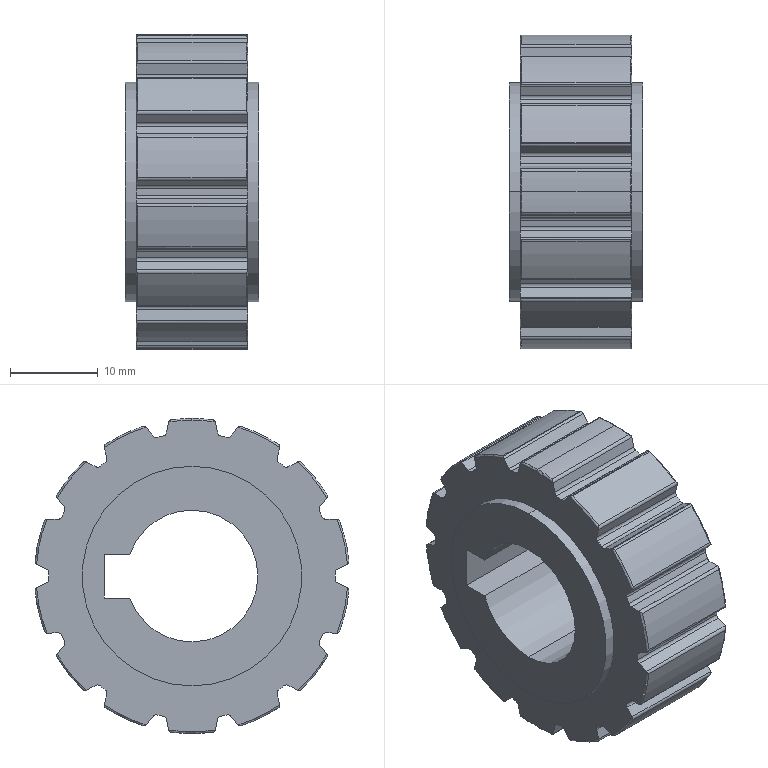Part | SolidWorks | features ICE 3, Cut 2, Chamfer 1, CirPattern 1, Fillet 1, RefAxis 1, Revolution 1 | 1 solid | 169 faces | box 15.24 x 35.738 x 35.892 mm | volume 10593 mm3 | cylinder 104 | plane 35 | torus 30 | commonest cylinder face diameters 0.76 x34 0.82 x34 35.892 x15 32.592 x14 25 x4 15 x3